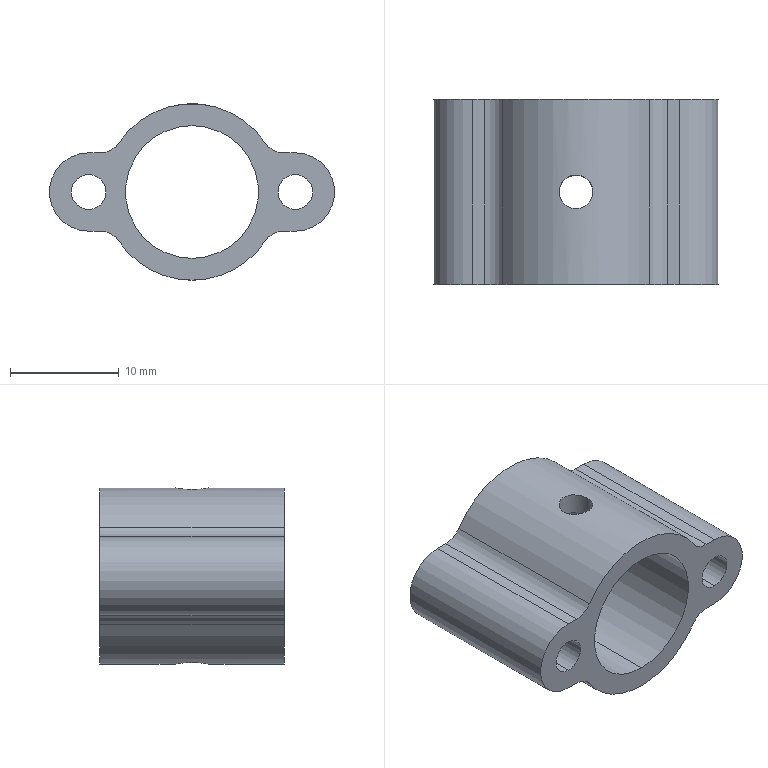Part | SolidWorks | features Extrusion 1, Fillet 1, ICE 1 | 1 solid | 25 faces | box 26.2 x 17 x 16.2 mm | volume 2329 mm3 | cylinder 19 | plane 6 | commonest cylinder face diameters 3.1 x4 3.2 x4 4 x4 16.2 x3 7.2 x2 12.2 x2
STEP:
#1=CARTESIAN_POINT('',(-1.55,8.5,-7.95));
#2=VERTEX_POINT('',#1);
#3=CARTESIAN_POINT('',(0.,6.95,-8.1));
#4=VERTEX_POINT('',#3);
#5=CARTESIAN_POINT('',(-1.55,8.5,-7.95));
#6=CARTESIAN_POINT('',(-1.55,8.398,-7.95));
#7=CARTESIAN_POINT('',(-1.54,8.297,-7.952));
#8=CARTESIAN_POINT('',(-1.5,8.098,-7.96));
#9=CARTESIAN_POINT('',(-1.471,8.,-7.965));
#10=CARTESIAN_POINT('',(-1.393,7.812,-7.979));
#11=CARTESIAN_POINT('',(-1.345,7.724,-7.988));
#12=CARTESIAN_POINT('',(-1.233,7.555,-8.006));
#13=CARTESIAN_POINT('',(-1.168,7.476,-8.016));
#14=CARTESIAN_POINT('',(-0.9541,7.262,-8.045));
#15=CARTESIAN_POINT('',(-0.7816,7.146,-8.064));
#16=CARTESIAN_POINT('',(-0.409,6.991,-8.092));
#17=CARTESIAN_POINT('',(-0.2052,6.95,-8.1));
#18=CARTESIAN_POINT('',(0.,6.95,-8.1));
#19=B_SPLINE_CURVE_WITH_KNOTS('',3,(#5,#6,#7,#8,#9,#10,#11,#12,#13,#14,#15,#16,#17,#18),.UNSPECIFIED.,.F.,.F.,(4,2,2,2,2,2,4),(0.007286,0.007589,0.007893,0.008196,0.0085,0.009106,0.009713),.UNSPECIFIED.);
#20=EDGE_CURVE('',#2,#4,#19,.T.);
#21=ORIENTED_EDGE('',*,*,#20,.F.);
#22=CARTESIAN_POINT('',(-1.55,8.5,-5.9));
#23=VERTEX_POINT('',#22);
#24=CARTESIAN_POINT('',(-1.55,8.5,-8.1));
#25=DIRECTION('',(0.,0.,1.));
#26=VECTOR('',#25,1000.);
#27=LINE('',#24,#26);
#28=EDGE_CURVE('',#2,#23,#27,.T.);
#29=ORIENTED_EDGE('',*,*,#28,.T.);
#30=CARTESIAN_POINT('',(0.,6.95,-6.1));
#31=VERTEX_POINT('',#30);
#32=CARTESIAN_POINT('',(-1.55,8.5,-5.9));
#33=CARTESIAN_POINT('',(-1.55,8.398,-5.9));
#34=CARTESIAN_POINT('',(-1.54,8.295,-5.903));
#35=CARTESIAN_POINT('',(-1.5,8.096,-5.913));
#36=CARTESIAN_POINT('',(-1.47,7.999,-5.92));
#37=CARTESIAN_POINT('',(-1.353,7.717,-5.949));
#38=CARTESIAN_POINT('',(-1.239,7.547,-5.975));
#39=CARTESIAN_POINT('',(-1.024,7.332,-6.014));
#40=CARTESIAN_POINT('',(-0.9459,7.268,-6.027));
#41=CARTESIAN_POINT('',(-0.7784,7.156,-6.051));
#42=CARTESIAN_POINT('',(-0.6876,7.107,-6.062));
#43=CARTESIAN_POINT('',(-0.5005,7.03,-6.08));
#44=CARTESIAN_POINT('',(-0.4039,7.,-6.087));
#45=CARTESIAN_POINT('',(-0.2043,6.96,-6.097));
#46=CARTESIAN_POINT('',(-0.1014,6.95,-6.1));
#47=CARTESIAN_POINT('',(0.,6.95,-6.1));
#48=B_SPLINE_CURVE_WITH_KNOTS('',3,(#32,#33,#34,#35,#36,#37,#38,#39,#40,#41,#42,#43,#44,#45,#46,#47),.UNSPECIFIED.,.F.,.F.,(4,2,2,2,2,2,2,4),(0.002434,0.002738,0.003042,0.00365,0.003954,0.004258,0.004562,0.004866),.UNSPECIFIED.);
#49=EDGE_CURVE('',#23,#31,#48,.T.);
#50=ORIENTED_EDGE('',*,*,#49,.T.);
#51=CARTESIAN_POINT('',(1.55,8.5,-5.9));
#52=VERTEX_POINT('',#51);
#53=CARTESIAN_POINT('',(0.,6.95,-6.1));
#54=CARTESIAN_POINT('',(0.2028,6.95,-6.1));
#55=CARTESIAN_POINT('',(0.4076,6.991,-6.089));
#56=CARTESIAN_POINT('',(0.6877,7.107,-6.062));
#57=CARTESIAN_POINT('',(0.7783,7.156,-6.051));
#58=CARTESIAN_POINT('',(0.9465,7.268,-6.027));
#59=CARTESIAN_POINT('',(1.024,7.332,-6.014));
#60=CARTESIAN_POINT('',(1.167,7.475,-5.988));
#61=CARTESIAN_POINT('',(1.232,7.554,-5.975));
#62=CARTESIAN_POINT('',(1.344,7.722,-5.95));
#63=CARTESIAN_POINT('',(1.392,7.811,-5.939));
#64=CARTESIAN_POINT('',(1.51,8.094,-5.911));
#65=CARTESIAN_POINT('',(1.55,8.296,-5.9));
#66=CARTESIAN_POINT('',(1.55,8.5,-5.9));
#67=B_SPLINE_CURVE_WITH_KNOTS('',3,(#53,#54,#55,#56,#57,#58,#59,#60,#61,#62,#63,#64,#65,#66),.UNSPECIFIED.,.F.,.F.,(4,2,2,2,2,2,4),(0.004866,0.005474,0.005778,0.006082,0.006387,0.006691,0.007299),.UNSPECIFIED.);
#68=EDGE_CURVE('',#31,#52,#67,.T.);
#69=ORIENTED_EDGE('',*,*,#68,.T.);
#70=CARTESIAN_POINT('',(1.55,8.5,-7.95));
#71=VERTEX_POINT('',#70);
#72=CARTESIAN_POINT('',(1.55,8.5,-8.1));
#73=DIRECTION('',(0.,0.,1.));
#74=VECTOR('',#73,1000.);
#75=LINE('',#72,#74);
#76=EDGE_CURVE('',#71,#52,#75,.T.);
#77=ORIENTED_EDGE('',*,*,#76,.F.);
#78=CARTESIAN_POINT('',(0.,6.95,-8.1));
#79=CARTESIAN_POINT('',(0.1027,6.95,-8.1));
#80=CARTESIAN_POINT('',(0.2036,6.96,-8.098));
#81=CARTESIAN_POINT('',(0.4021,7.,-8.091));
#82=CARTESIAN_POINT('',(0.5007,7.03,-8.085));
#83=CARTESIAN_POINT('',(0.6884,7.108,-8.071));
#84=CARTESIAN_POINT('',(0.7773,7.155,-8.063));
#85=CARTESIAN_POINT('',(0.9457,7.268,-8.045));
#86=CARTESIAN_POINT('',(1.025,7.333,-8.035));
#87=CARTESIAN_POINT('',(1.239,7.547,-8.006));
#88=CARTESIAN_POINT('',(1.354,7.72,-7.986));
#89=CARTESIAN_POINT('',(1.509,8.093,-7.959));
#90=CARTESIAN_POINT('',(1.55,8.297,-7.95));
#91=CARTESIAN_POINT('',(1.55,8.5,-7.95));
#92=B_SPLINE_CURVE_WITH_KNOTS('',3,(#78,#79,#80,#81,#82,#83,#84,#85,#86,#87,#88,#89,#90,#91),.UNSPECIFIED.,.F.,.F.,(4,2,2,2,2,2,4),(0.,0.0003037,0.0006073,0.000911,0.001215,0.001822,0.002429),.UNSPECIFIED.);
#93=EDGE_CURVE('',#4,#71,#92,.T.);
#94=ORIENTED_EDGE('',*,*,#93,.F.);
#95=EDGE_LOOP('',(#21,#29,#50,#69,#77,#94));
#96=FACE_OUTER_BOUND('',#95,.T.);
#97=CARTESIAN_POINT('',(0.,8.5,-8.1));
#98=DIRECTION('',(0.,0.,1.));
#99=DIRECTION('',(1.,0.,0.));
#100=AXIS2_PLACEMENT_3D('',#97,#98,#99);
#101=CYLINDRICAL_SURFACE('',#100,1.55);
#102=ADVANCED_FACE('',(#96),#101,.F.);
#103=CARTESIAN_POINT('',(0.,6.95,6.1));
#104=VERTEX_POINT('',#103);
#105=CARTESIAN_POINT('',(-1.55,8.5,5.9));
#106=VERTEX_POINT('',#105);
#107=CARTESIAN_POINT('',(0.,6.95,6.1));
#108=CARTESIAN_POINT('',(-0.1016,6.95,6.1));
#109=CARTESIAN_POINT('',(-0.2047,6.96,6.097));
#110=CARTESIAN_POINT('',(-0.4038,7.,6.087));
#111=CARTESIAN_POINT('',(-0.5006,7.03,6.08));
#112=CARTESIAN_POINT('',(-0.7828,7.147,6.053));
#113=CARTESIAN_POINT('',(-0.9531,7.261,6.027));
#114=CARTESIAN_POINT('',(-1.168,7.476,5.988));
#115=CARTESIAN_POINT('',(-1.232,7.554,5.975));
#116=CARTESIAN_POINT('',(-1.344,7.722,5.95));
#117=CARTESIAN_POINT('',(-1.393,7.812,5.939));
#118=CARTESIAN_POINT('',(-1.47,7.999,5.92));
#119=CARTESIAN_POINT('',(-1.5,8.096,5.913));
#120=CARTESIAN_POINT('',(-1.54,8.296,5.902));
#121=CARTESIAN_POINT('',(-1.55,8.399,5.9));
#122=CARTESIAN_POINT('',(-1.55,8.5,5.9));
#123=B_SPLINE_CURVE_WITH_KNOTS('',3,(#107,#108,#109,#110,#111,#112,#113,#114,#115,#116,#117,#118,#119,#120,#121,#122),.UNSPECIFIED.,.F.,.F.,(4,2,2,2,2,2,2,4),(0.002434,0.002738,0.003042,0.00365,0.003954,0.004258,0.004562,0.004866),.UNSPECIFIED.);
#124=EDGE_CURVE('',#104,#106,#123,.T.);
#125=ORIENTED_EDGE('',*,*,#124,.T.);
#126=CARTESIAN_POINT('',(-1.55,8.5,7.95));
#127=VERTEX_POINT('',#126);
#128=CARTESIAN_POINT('',(-1.55,8.5,-8.1));
#129=DIRECTION('',(0.,0.,1.));
#130=VECTOR('',#129,1000.);
#131=LINE('',#128,#130);
#132=EDGE_CURVE('',#106,#127,#131,.T.);
#133=ORIENTED_EDGE('',*,*,#132,.T.);
#134=CARTESIAN_POINT('',(1.55,8.5,7.95));
#135=VERTEX_POINT('',#134);
#136=CARTESIAN_POINT('',(1.55,8.5,7.95));
#137=CARTESIAN_POINT('',(1.55,8.397,7.95));
#138=CARTESIAN_POINT('',(1.54,8.296,7.952));
#139=CARTESIAN_POINT('',(1.5,8.098,7.96));
#140=CARTESIAN_POINT('',(1.47,7.999,7.966));
#141=CARTESIAN_POINT('',(1.393,7.812,7.979));
#142=CARTESIAN_POINT('',(1.345,7.723,7.988));
#143=CARTESIAN_POINT('',(1.232,7.555,8.006));
#144=CARTESIAN_POINT('',(1.167,7.475,8.016));
#145=CARTESIAN_POINT('',(0.9531,7.261,8.045));
#146=CARTESIAN_POINT('',(0.7805,7.146,8.064));
#147=CARTESIAN_POINT('',(0.4076,6.991,8.092));
#148=CARTESIAN_POINT('',(0.2033,6.95,8.1));
#149=CARTESIAN_POINT('',(-0.1008,6.95,8.1));
#150=CARTESIAN_POINT('',(-0.2037,6.96,8.098));
#151=CARTESIAN_POINT('',(-0.4027,7.,8.091));
#152=CARTESIAN_POINT('',(-0.4995,7.029,8.085));
#153=CARTESIAN_POINT('',(-0.7814,7.146,8.064));
#154=CARTESIAN_POINT('',(-0.952,7.26,8.045));
#155=CARTESIAN_POINT('',(-1.168,7.476,8.016));
#156=CARTESIAN_POINT('',(-1.232,7.554,8.006));
#157=CARTESIAN_POINT('',(-1.344,7.722,7.988));
#158=CARTESIAN_POINT('',(-1.393,7.813,7.979));
#159=CARTESIAN_POINT('',(-1.471,8.,7.965));
#160=CARTESIAN_POINT('',(-1.5,8.097,7.96));
#161=CARTESIAN_POINT('',(-1.54,8.296,7.952));
#162=CARTESIAN_POINT('',(-1.55,8.399,7.95));
#163=CARTESIAN_POINT('',(-1.55,8.5,7.95));
#164=B_SPLINE_CURVE_WITH_KNOTS('',3,(#136,#137,#138,#139,#140,#141,#142,#143,#144,#145,#146,#147,#148,#149,#150,#151,#152,#153,#154,#155,#156,#157,#158,#159,#160,#161,#162,#163),.UNSPECIFIED.,.F.,.F.,(4,2,2,2,2,2,2,2,2,2,2,2,2,4),(0.,0.0003036,0.0006072,0.0009107,0.001214,0.001821,0.002429,0.002732,0.003036,0.003643,0.003946,0.00425,0.004554,0.004857),.UNSPECIFIED.);
#165=EDGE_CURVE('',#135,#127,#164,.T.);
#166=ORIENTED_EDGE('',*,*,#165,.F.);
#167=CARTESIAN_POINT('',(1.55,8.5,5.9));
#168=VERTEX_POINT('',#167);
#169=CARTESIAN_POINT('',(1.55,8.5,-8.1));
#170=DIRECTION('',(0.,0.,1.));
#171=VECTOR('',#170,1000.);
#172=LINE('',#169,#171);
#173=EDGE_CURVE('',#168,#135,#172,.T.);
#174=ORIENTED_EDGE('',*,*,#173,.F.);
#175=CARTESIAN_POINT('',(1.55,8.5,5.9));
#176=CARTESIAN_POINT('',(1.55,8.397,5.9));
#177=CARTESIAN_POINT('',(1.54,8.296,5.902));
#178=CARTESIAN_POINT('',(1.5,8.097,5.913));
#179=CARTESIAN_POINT('',(1.47,7.999,5.92));
#180=CARTESIAN_POINT('',(1.392,7.811,5.939));
#181=CARTESIAN_POINT('',(1.345,7.722,5.95));
#182=CARTESIAN_POINT('',(1.232,7.554,5.975));
#183=CARTESIAN_POINT('',(1.167,7.475,5.988));
#184=CARTESIAN_POINT('',(0.9531,7.261,6.027));
#185=CARTESIAN_POINT('',(0.7807,7.146,6.053));
#186=CARTESIAN_POINT('',(0.4078,6.991,6.089));
#187=CARTESIAN_POINT('',(0.2032,6.95,6.1));
#188=CARTESIAN_POINT('',(0.,6.95,6.1));
#189=B_SPLINE_CURVE_WITH_KNOTS('',3,(#175,#176,#177,#178,#179,#180,#181,#182,#183,#184,#185,#186,#187,#188),.UNSPECIFIED.,.F.,.F.,(4,2,2,2,2,2,4),(0.,0.0003042,0.0006084,0.0009126,0.001217,0.001825,0.002434),.UNSPECIFIED.);
#190=EDGE_CURVE('',#168,#104,#189,.T.);
#191=ORIENTED_EDGE('',*,*,#190,.T.);
#192=EDGE_LOOP('',(#125,#133,#166,#174,#191));
#193=FACE_OUTER_BOUND('',#192,.T.);
#194=CARTESIAN_POINT('',(0.,8.5,-8.1));
#195=DIRECTION('',(0.,0.,1.));
#196=DIRECTION('',(1.,0.,0.));
#197=AXIS2_PLACEMENT_3D('',#194,#195,#196);
#198=CYLINDRICAL_SURFACE('',#197,1.55);
#199=ADVANCED_FACE('',(#193),#198,.F.);
#200=CARTESIAN_POINT('',(-9.5,17.,-1.6));
#201=VERTEX_POINT('',#200);
#202=CARTESIAN_POINT('',(-9.5,17.,1.6));
#203=VERTEX_POINT('',#202);
#204=CARTESIAN_POINT('',(-9.5,17.,0.));
#205=DIRECTION('',(0.,1.,0.));
#206=DIRECTION('',(0.,0.,-1.));
#207=AXIS2_PLACEMENT_3D('',#204,#205,#206);
#208=CIRCLE('',#207,1.6);
#209=EDGE_CURVE('',#201,#203,#208,.T.);
#210=ORIENTED_EDGE('',*,*,#209,.T.);
#211=CARTESIAN_POINT('',(-9.5,0.,1.6));
#212=VERTEX_POINT('',#211);
#213=CARTESIAN_POINT('',(-9.5,17.,1.6));
#214=DIRECTION('',(0.,-1.,0.));
#215=VECTOR('',#214,1000.);
#216=LINE('',#213,#215);
#217=EDGE_CURVE('',#203,#212,#216,.T.);
#218=ORIENTED_EDGE('',*,*,#217,.T.);
#219=CARTESIAN_POINT('',(-9.5,0.,-1.6));
#220=VERTEX_POINT('',#219);
#221=CARTESIAN_POINT('',(-9.5,0.,0.));
#222=DIRECTION('',(0.,1.,0.));
#223=DIRECTION('',(0.,0.,-1.));
#224=AXIS2_PLACEMENT_3D('',#221,#222,#223);
#225=CIRCLE('',#224,1.6);
#226=EDGE_CURVE('',#220,#212,#225,.T.);
#227=ORIENTED_EDGE('',*,*,#226,.F.);
#228=CARTESIAN_POINT('',(-9.5,17.,-1.6));
#229=DIRECTION('',(0.,-1.,0.));
#230=VECTOR('',#229,1000.);
#231=LINE('',#228,#230);
#232=EDGE_CURVE('',#201,#220,#231,.T.);
#233=ORIENTED_EDGE('',*,*,#232,.F.);
#234=EDGE_LOOP('',(#210,#218,#227,#233));
#235=FACE_OUTER_BOUND('',#234,.T.);
#236=CARTESIAN_POINT('',(-9.5,17.,0.));
#237=DIRECTION('',(0.,-1.,0.));
#238=DIRECTION('',(0.,0.,-1.));
#239=AXIS2_PLACEMENT_3D('',#236,#237,#238);
#240=CYLINDRICAL_SURFACE('',#239,1.6);
#241=ADVANCED_FACE('',(#235),#240,.F.);
#242=CARTESIAN_POINT('',(9.5,17.,-1.6));
#243=VERTEX_POINT('',#242);
#244=CARTESIAN_POINT('',(9.5,17.,1.6));
#245=VERTEX_POINT('',#244);
#246=CARTESIAN_POINT('',(9.5,17.,0.));
#247=DIRECTION('',(0.,1.,0.));
#248=DIRECTION('',(0.,0.,1.));
#249=AXIS2_PLACEMENT_3D('',#246,#247,#248);
#250=CIRCLE('',#249,1.6);
#251=EDGE_CURVE('',#243,#245,#250,.T.);
#252=ORIENTED_EDGE('',*,*,#251,.T.);
#253=CARTESIAN_POINT('',(9.5,0.,1.6));
#254=VERTEX_POINT('',#253);
#255=CARTESIAN_POINT('',(9.5,17.,1.6));
#256=DIRECTION('',(0.,-1.,0.));
#257=VECTOR('',#256,1000.);
#258=LINE('',#255,#257);
#259=EDGE_CURVE('',#245,#254,#258,.T.);
#260=ORIENTED_EDGE('',*,*,#259,.T.);
#261=CARTESIAN_POINT('',(9.5,0.,-1.6));
#262=VERTEX_POINT('',#261);
#263=CARTESIAN_POINT('',(9.5,0.,0.));
#264=DIRECTION('',(0.,1.,0.));
#265=DIRECTION('',(0.,0.,1.));
#266=AXIS2_PLACEMENT_3D('',#263,#264,#265);
#267=CIRCLE('',#266,1.6);
#268=EDGE_CURVE('',#262,#254,#267,.T.);
#269=ORIENTED_EDGE('',*,*,#268,.F.);
#270=CARTESIAN_POINT('',(9.5,17.,-1.6));
#271=DIRECTION('',(0.,-1.,0.));
#272=VECTOR('',#271,1000.);
#273=LINE('',#270,#272);
#274=EDGE_CURVE('',#243,#262,#273,.T.);
#275=ORIENTED_EDGE('',*,*,#274,.F.);
#276=EDGE_LOOP('',(#252,#260,#269,#275));
#277=FACE_OUTER_BOUND('',#276,.T.);
#278=CARTESIAN_POINT('',(9.5,17.,0.));
#279=DIRECTION('',(0.,-1.,0.));
#280=DIRECTION('',(0.,0.,-1.));
#281=AXIS2_PLACEMENT_3D('',#278,#279,#280);
#282=CYLINDRICAL_SURFACE('',#281,1.6);
#283=ADVANCED_FACE('',(#277),#282,.F.);
#284=CARTESIAN_POINT('',(0.,17.,-6.1));
#285=VERTEX_POINT('',#284);
#286=CARTESIAN_POINT('',(0.,17.,6.1));
#287=VERTEX_POINT('',#286);
#288=CARTESIAN_POINT('',(0.,17.,0.));
#289=DIRECTION('',(0.,1.,0.));
#290=DIRECTION('',(0.,0.,1.));
#291=AXIS2_PLACEMENT_3D('',#288,#289,#290);
#292=CIRCLE('',#291,6.1);
#293=EDGE_CURVE('',#285,#287,#292,.T.);
#294=ORIENTED_EDGE('',*,*,#293,.T.);
#295=CARTESIAN_POINT('',(0.,10.05,6.1));
#296=VERTEX_POINT('',#295);
#297=CARTESIAN_POINT('',(0.,17.,6.1));
#298=DIRECTION('',(0.,-1.,0.));
#299=VECTOR('',#298,1000.);
#300=LINE('',#297,#299);
#301=EDGE_CURVE('',#287,#296,#300,.T.);
#302=ORIENTED_EDGE('',*,*,#301,.T.);
#303=CARTESIAN_POINT('',(-1.55,8.5,5.9));
#304=CARTESIAN_POINT('',(-1.55,8.703,5.9));
#305=CARTESIAN_POINT('',(-1.509,8.908,5.911));
#306=CARTESIAN_POINT('',(-1.393,9.188,5.939));
#307=CARTESIAN_POINT('',(-1.344,9.278,5.95));
#308=CARTESIAN_POINT('',(-1.232,9.446,5.975));
#309=CARTESIAN_POINT('',(-1.168,9.524,5.988));
#310=CARTESIAN_POINT('',(-1.025,9.667,6.014));
#311=CARTESIAN_POINT('',(-0.9456,9.732,6.027));
#312=CARTESIAN_POINT('',(-0.7782,9.844,6.051));
#313=CARTESIAN_POINT('',(-0.6893,9.892,6.062));
#314=CARTESIAN_POINT('',(-0.4063,10.01,6.089));
#315=CARTESIAN_POINT('',(-0.2045,10.05,6.1));
#316=CARTESIAN_POINT('',(0.,10.05,6.1));
#317=B_SPLINE_CURVE_WITH_KNOTS('',3,(#303,#304,#305,#306,#307,#308,#309,#310,#311,#312,#313,#314,#315,#316),.UNSPECIFIED.,.F.,.F.,(4,2,2,2,2,2,4),(0.004866,0.005474,0.005778,0.006082,0.006386,0.006691,0.007299),.UNSPECIFIED.);
#318=EDGE_CURVE('',#106,#296,#317,.T.);
#319=ORIENTED_EDGE('',*,*,#318,.F.);
#320=ORIENTED_EDGE('',*,*,#124,.F.);
#321=CARTESIAN_POINT('',(0.,0.,6.1));
#322=VERTEX_POINT('',#321);
#323=CARTESIAN_POINT('',(0.,17.,6.1));
#324=DIRECTION('',(0.,-1.,0.));
#325=VECTOR('',#324,1000.);
#326=LINE('',#323,#325);
#327=EDGE_CURVE('',#104,#322,#326,.T.);
#328=ORIENTED_EDGE('',*,*,#327,.T.);
#329=CARTESIAN_POINT('',(0.,0.,-6.1));
#330=VERTEX_POINT('',#329);
#331=CARTESIAN_POINT('',(0.,0.,0.));
#332=DIRECTION('',(0.,1.,0.));
#333=DIRECTION('',(0.,0.,1.));
#334=AXIS2_PLACEMENT_3D('',#331,#332,#333);
#335=CIRCLE('',#334,6.1);
#336=EDGE_CURVE('',#330,#322,#335,.T.);
#337=ORIENTED_EDGE('',*,*,#336,.F.);
#338=CARTESIAN_POINT('',(0.,17.,-6.1));
#339=DIRECTION('',(0.,-1.,0.));
#340=VECTOR('',#339,1000.);
#341=LINE('',#338,#340);
#342=EDGE_CURVE('',#31,#330,#341,.T.);
#343=ORIENTED_EDGE('',*,*,#342,.F.);
#344=ORIENTED_EDGE('',*,*,#49,.F.);
#345=CARTESIAN_POINT('',(0.,10.05,-6.1));
#346=VERTEX_POINT('',#345);
#347=CARTESIAN_POINT('',(0.,10.05,-6.1));
#348=CARTESIAN_POINT('',(-0.1029,10.05,-6.1));
#349=CARTESIAN_POINT('',(-0.204,10.04,-6.097));
#350=CARTESIAN_POINT('',(-0.4027,10.,-6.088));
#351=CARTESIAN_POINT('',(-0.5015,9.97,-6.08));
#352=CARTESIAN_POINT('',(-0.689,9.892,-6.062));
#353=CARTESIAN_POINT('',(-0.7779,9.844,-6.051));
#354=CARTESIAN_POINT('',(-0.9461,9.732,-6.027));
#355=CARTESIAN_POINT('',(-1.025,9.667,-6.014));
#356=CARTESIAN_POINT('',(-1.239,9.453,-5.975));
#357=CARTESIAN_POINT('',(-1.354,9.281,-5.948));
#358=CARTESIAN_POINT('',(-1.509,8.908,-5.911));
#359=CARTESIAN_POINT('',(-1.55,8.703,-5.9));
#360=CARTESIAN_POINT('',(-1.55,8.5,-5.9));
#361=B_SPLINE_CURVE_WITH_KNOTS('',3,(#347,#348,#349,#350,#351,#352,#353,#354,#355,#356,#357,#358,#359,#360),.UNSPECIFIED.,.F.,.F.,(4,2,2,2,2,2,4),(0.,0.0003042,0.0006084,0.0009126,0.001217,0.001825,0.002434),.UNSPECIFIED.);
#362=EDGE_CURVE('',#346,#23,#361,.T.);
#363=ORIENTED_EDGE('',*,*,#362,.F.);
#364=CARTESIAN_POINT('',(0.,17.,-6.1));
#365=DIRECTION('',(0.,-1.,0.));
#366=VECTOR('',#365,1000.);
#367=LINE('',#364,#366);
#368=EDGE_CURVE('',#285,#346,#367,.T.);
#369=ORIENTED_EDGE('',*,*,#368,.F.);
#370=EDGE_LOOP('',(#294,#302,#319,#320,#328,#337,#343,#344,#363,#369));
#371=FACE_OUTER_BOUND('',#370,.T.);
#372=CARTESIAN_POINT('',(0.,17.,0.));
#373=DIRECTION('',(0.,-1.,0.));
#374=DIRECTION('',(0.,0.,-1.));
#375=AXIS2_PLACEMENT_3D('',#372,#373,#374);
#376=CYLINDRICAL_SURFACE('',#375,6.1);
#377=ADVANCED_FACE('',(#371),#376,.F.);
#378=CARTESIAN_POINT('',(0.,17.,-8.1));
#379=VERTEX_POINT('',#378);
#380=CARTESIAN_POINT('',(-6.741,17.,-4.491));
#381=VERTEX_POINT('',#380);
#382=CARTESIAN_POINT('',(0.,17.,0.));
#383=DIRECTION('',(0.,1.,0.));
#384=DIRECTION('',(0.,0.,1.));
#385=AXIS2_PLACEMENT_3D('',#382,#383,#384);
#386=CIRCLE('',#385,8.1);
#387=EDGE_CURVE('',#379,#381,#386,.T.);
#388=ORIENTED_EDGE('',*,*,#387,.F.);
#389=CARTESIAN_POINT('',(0.,10.05,-8.1));
#390=VERTEX_POINT('',#389);
#391=CARTESIAN_POINT('',(0.,17.,-8.1));
#392=DIRECTION('',(0.,-1.,0.));
#393=VECTOR('',#392,1000.);
#394=LINE('',#391,#393);
#395=EDGE_CURVE('',#379,#390,#394,.T.);
#396=ORIENTED_EDGE('',*,*,#395,.T.);
#397=CARTESIAN_POINT('',(0.,10.05,-8.1));
#398=CARTESIAN_POINT('',(-0.2026,10.05,-8.1));
#399=CARTESIAN_POINT('',(-0.407,10.009,-8.092));
#400=CARTESIAN_POINT('',(-0.7803,9.854,-8.064));
#401=CARTESIAN_POINT('',(-0.9527,9.739,-8.045));
#402=CARTESIAN_POINT('',(-1.167,9.525,-8.016));
#403=CARTESIAN_POINT('',(-1.232,9.445,-8.006));
#404=CARTESIAN_POINT('',(-1.345,9.277,-7.988));
#405=CARTESIAN_POINT('',(-1.392,9.188,-7.98));
#406=CARTESIAN_POINT('',(-1.51,8.906,-7.958));
#407=CARTESIAN_POINT('',(-1.55,8.705,-7.95));
#408=CARTESIAN_POINT('',(-1.55,8.5,-7.95));
#409=B_SPLINE_CURVE_WITH_KNOTS('',3,(#397,#398,#399,#400,#401,#402,#403,#404,#405,#406,#407,#408),.UNSPECIFIED.,.F.,.F.,(4,2,2,2,2,4),(0.004857,0.005464,0.006072,0.006375,0.006679,0.007286),.UNSPECIFIED.);
#410=EDGE_CURVE('',#390,#2,#409,.T.);
#411=ORIENTED_EDGE('',*,*,#410,.T.);
#412=ORIENTED_EDGE('',*,*,#20,.T.);
#413=CARTESIAN_POINT('',(0.,0.,-8.1));
#414=VERTEX_POINT('',#413);
#415=CARTESIAN_POINT('',(0.,17.,-8.1));
#416=DIRECTION('',(0.,-1.,0.));
#417=VECTOR('',#416,1000.);
#418=LINE('',#415,#417);
#419=EDGE_CURVE('',#4,#414,#418,.T.);
#420=ORIENTED_EDGE('',*,*,#419,.T.);
#421=CARTESIAN_POINT('',(-6.741,0.,-4.491));
#422=VERTEX_POINT('',#421);
#423=CARTESIAN_POINT('',(0.,0.,0.));
#424=DIRECTION('',(0.,1.,0.));
#425=DIRECTION('',(0.,0.,1.));
#426=AXIS2_PLACEMENT_3D('',#423,#424,#425);
#427=CIRCLE('',#426,8.1);
#428=EDGE_CURVE('',#414,#422,#427,.T.);
#429=ORIENTED_EDGE('',*,*,#428,.T.);
#430=CARTESIAN_POINT('',(-6.741,17.,-4.491));
#431=DIRECTION('',(0.,1.,0.));
#432=VECTOR('',#431,1000.);
#433=LINE('',#430,#432);
#434=EDGE_CURVE('',#422,#381,#433,.T.);
#435=ORIENTED_EDGE('',*,*,#434,.T.);
#436=EDGE_LOOP('',(#388,#396,#411,#412,#420,#429,#435));
#437=FACE_OUTER_BOUND('',#436,.T.);
#438=CARTESIAN_POINT('',(0.,17.,0.));
#439=DIRECTION('',(0.,-1.,0.));
#440=DIRECTION('',(0.,0.,-1.));
#441=AXIS2_PLACEMENT_3D('',#438,#439,#440);
#442=CYLINDRICAL_SURFACE('',#441,8.1);
#443=ADVANCED_FACE('',(#437),#442,.T.);
#444=CARTESIAN_POINT('',(-9.5,17.,-3.6));
#445=VERTEX_POINT('',#444);
#446=CARTESIAN_POINT('',(-9.5,17.,3.6));
#447=VERTEX_POINT('',#446);
#448=CARTESIAN_POINT('',(-9.5,17.,0.));
#449=DIRECTION('',(0.,1.,0.));
#450=DIRECTION('',(0.,0.,-1.));
#451=AXIS2_PLACEMENT_3D('',#448,#449,#450);
#452=CIRCLE('',#451,3.6);
#453=EDGE_CURVE('',#445,#447,#452,.T.);
#454=ORIENTED_EDGE('',*,*,#453,.T.);
#455=CARTESIAN_POINT('',(-8.405,17.,3.6));
#456=VERTEX_POINT('',#455);
#457=CARTESIAN_POINT('',(-9.5,17.,3.6));
#458=DIRECTION('',(1.,0.,0.));
#459=VECTOR('',#458,1000.);
#460=LINE('',#457,#459);
#461=EDGE_CURVE('',#447,#456,#460,.T.);
#462=ORIENTED_EDGE('',*,*,#461,.T.);
#463=CARTESIAN_POINT('',(-6.741,17.,4.491));
#464=VERTEX_POINT('',#463);
#465=CARTESIAN_POINT('',(-8.405,17.,5.6));
#466=DIRECTION('',(0.,-1.,0.));
#467=DIRECTION('',(0.,0.,-1.));
#468=AXIS2_PLACEMENT_3D('',#465,#466,#467);
#469=CIRCLE('',#468,2.);
#470=EDGE_CURVE('',#456,#464,#469,.T.);
#471=ORIENTED_EDGE('',*,*,#470,.T.);
#472=CARTESIAN_POINT('',(6.741,17.,4.491));
#473=VERTEX_POINT('',#472);
#474=CARTESIAN_POINT('',(0.,17.,0.));
#475=DIRECTION('',(0.,1.,0.));
#476=DIRECTION('',(0.,0.,1.));
#477=AXIS2_PLACEMENT_3D('',#474,#475,#476);
#478=CIRCLE('',#477,8.1);
#479=EDGE_CURVE('',#464,#473,#478,.T.);
#480=ORIENTED_EDGE('',*,*,#479,.T.);
#481=CARTESIAN_POINT('',(8.405,17.,3.6));
#482=VERTEX_POINT('',#481);
#483=CARTESIAN_POINT('',(8.405,17.,5.6));
#484=DIRECTION('',(0.,-1.,0.));
#485=DIRECTION('',(0.,0.,-1.));
#486=AXIS2_PLACEMENT_3D('',#483,#484,#485);
#487=CIRCLE('',#486,2.);
#488=EDGE_CURVE('',#473,#482,#487,.T.);
#489=ORIENTED_EDGE('',*,*,#488,.T.);
#490=CARTESIAN_POINT('',(9.5,17.,3.6));
#491=VERTEX_POINT('',#490);
#492=CARTESIAN_POINT('',(9.5,17.,3.6));
#493=DIRECTION('',(1.,0.,0.));
#494=VECTOR('',#493,1000.);
#495=LINE('',#492,#494);
#496=EDGE_CURVE('',#482,#491,#495,.T.);
#497=ORIENTED_EDGE('',*,*,#496,.T.);
#498=CARTESIAN_POINT('',(9.5,17.,-3.6));
#499=VERTEX_POINT('',#498);
#500=CARTESIAN_POINT('',(9.5,17.,0.));
#501=DIRECTION('',(0.,1.,0.));
#502=DIRECTION('',(0.,0.,1.));
#503=AXIS2_PLACEMENT_3D('',#500,#501,#502);
#504=CIRCLE('',#503,3.6);
#505=EDGE_CURVE('',#491,#499,#504,.T.);
#506=ORIENTED_EDGE('',*,*,#505,.T.);
#507=CARTESIAN_POINT('',(8.405,17.,-3.6));
#508=VERTEX_POINT('',#507);
#509=CARTESIAN_POINT('',(9.5,17.,-3.6));
#510=DIRECTION('',(-1.,0.,0.));
#511=VECTOR('',#510,1000.);
#512=LINE('',#509,#511);
#513=EDGE_CURVE('',#499,#508,#512,.T.);
#514=ORIENTED_EDGE('',*,*,#513,.T.);
#515=CARTESIAN_POINT('',(6.741,17.,-4.491));
#516=VERTEX_POINT('',#515);
#517=CARTESIAN_POINT('',(8.405,17.,-5.6));
#518=DIRECTION('',(0.,-1.,0.));
#519=DIRECTION('',(0.,0.,-1.));
#520=AXIS2_PLACEMENT_3D('',#517,#518,#519);
#521=CIRCLE('',#520,2.);
#522=EDGE_CURVE('',#508,#516,#521,.T.);
#523=ORIENTED_EDGE('',*,*,#522,.T.);
#524=CARTESIAN_POINT('',(0.,17.,0.));
#525=DIRECTION('',(0.,1.,0.));
#526=DIRECTION('',(0.,0.,1.));
#527=AXIS2_PLACEMENT_3D('',#524,#525,#526);
#528=CIRCLE('',#527,8.1);
#529=EDGE_CURVE('',#516,#379,#528,.T.);
#530=ORIENTED_EDGE('',*,*,#529,.T.);
#531=ORIENTED_EDGE('',*,*,#387,.T.);
#532=CARTESIAN_POINT('',(-8.405,17.,-3.6));
#533=VERTEX_POINT('',#532);
#534=CARTESIAN_POINT('',(-8.405,17.,-5.6));
#535=DIRECTION('',(0.,-1.,0.));
#536=DIRECTION('',(0.,0.,-1.));
#537=AXIS2_PLACEMENT_3D('',#534,#535,#536);
#538=CIRCLE('',#537,2.);
#539=EDGE_CURVE('',#381,#533,#538,.T.);
#540=ORIENTED_EDGE('',*,*,#539,.T.);
#541=CARTESIAN_POINT('',(-9.5,17.,-3.6));
#542=DIRECTION('',(-1.,0.,0.));
#543=VECTOR('',#542,1000.);
#544=LINE('',#541,#543);
#545=EDGE_CURVE('',#533,#445,#544,.T.);
#546=ORIENTED_EDGE('',*,*,#545,.T.);
#547=EDGE_LOOP('',(#454,#462,#471,#480,#489,#497,#506,#514,#523,#530,#531,#540,#546));
#548=FACE_OUTER_BOUND('',#547,.T.);
#549=ORIENTED_EDGE('',*,*,#293,.F.);
#550=CARTESIAN_POINT('',(0.,17.,0.));
#551=DIRECTION('',(0.,1.,0.));
#552=DIRECTION('',(0.,0.,1.));
#553=AXIS2_PLACEMENT_3D('',#550,#551,#552);
#554=CIRCLE('',#553,6.1);
#555=EDGE_CURVE('',#287,#285,#554,.T.);
#556=ORIENTED_EDGE('',*,*,#555,.F.);
#557=EDGE_LOOP('',(#549,#556));
#558=FACE_BOUND('',#557,.T.);
#559=ORIENTED_EDGE('',*,*,#251,.F.);
#560=CARTESIAN_POINT('',(9.5,17.,0.));
#561=DIRECTION('',(0.,1.,0.));
#562=DIRECTION('',(0.,0.,1.));
#563=AXIS2_PLACEMENT_3D('',#560,#561,#562);
#564=CIRCLE('',#563,1.6);
#565=EDGE_CURVE('',#245,#243,#564,.T.);
#566=ORIENTED_EDGE('',*,*,#565,.F.);
#567=EDGE_LOOP('',(#559,#566));
#568=FACE_BOUND('',#567,.T.);
#569=ORIENTED_EDGE('',*,*,#209,.F.);
#570=CARTESIAN_POINT('',(-9.5,17.,0.));
#571=DIRECTION('',(0.,1.,0.));
#572=DIRECTION('',(0.,0.,-1.));
#573=AXIS2_PLACEMENT_3D('',#570,#571,#572);
#574=CIRCLE('',#573,1.6);
#575=EDGE_CURVE('',#203,#201,#574,.T.);
#576=ORIENTED_EDGE('',*,*,#575,.F.);
#577=EDGE_LOOP('',(#569,#576));
#578=FACE_BOUND('',#577,.T.);
#579=CARTESIAN_POINT('',(-9.5,17.,0.));
#580=DIRECTION('',(0.,-1.,0.));
#581=DIRECTION('',(0.,0.,-1.));
#582=AXIS2_PLACEMENT_3D('',#579,#580,#581);
#583=PLANE('',#582);
#584=ADVANCED_FACE('',(#548,#558,#568,#578),#583,.F.);
#585=ORIENTED_EDGE('',*,*,#268,.T.);
#586=CARTESIAN_POINT('',(9.5,0.,0.));
#587=DIRECTION('',(0.,1.,0.));
#588=DIRECTION('',(0.,0.,1.));
#589=AXIS2_PLACEMENT_3D('',#586,#587,#588);
#590=CIRCLE('',#589,1.6);
#591=EDGE_CURVE('',#254,#262,#590,.T.);
#592=ORIENTED_EDGE('',*,*,#591,.T.);
#593=EDGE_LOOP('',(#585,#592));
#594=FACE_BOUND('',#593,.T.);
#595=CARTESIAN_POINT('',(-9.5,0.,-3.6));
#596=VERTEX_POINT('',#595);
#597=CARTESIAN_POINT('',(-9.5,0.,3.6));
#598=VERTEX_POINT('',#597);
#599=CARTESIAN_POINT('',(-9.5,0.,0.));
#600=DIRECTION('',(0.,1.,0.));
#601=DIRECTION('',(0.,0.,-1.));
#602=AXIS2_PLACEMENT_3D('',#599,#600,#601);
#603=CIRCLE('',#602,3.6);
#604=EDGE_CURVE('',#596,#598,#603,.T.);
#605=ORIENTED_EDGE('',*,*,#604,.F.);
#606=CARTESIAN_POINT('',(-8.405,0.,-3.6));
#607=VERTEX_POINT('',#606);
#608=CARTESIAN_POINT('',(-9.5,0.,-3.6));
#609=DIRECTION('',(-1.,0.,0.));
#610=VECTOR('',#609,1000.);
#611=LINE('',#608,#610);
#612=EDGE_CURVE('',#607,#596,#611,.T.);
#613=ORIENTED_EDGE('',*,*,#612,.F.);
#614=CARTESIAN_POINT('',(-8.405,0.,-5.6));
#615=DIRECTION('',(0.,1.,0.));
#616=DIRECTION('',(0.,0.,-1.));
#617=AXIS2_PLACEMENT_3D('',#614,#615,#616);
#618=CIRCLE('',#617,2.);
#619=EDGE_CURVE('',#607,#422,#618,.T.);
#620=ORIENTED_EDGE('',*,*,#619,.T.);
#621=ORIENTED_EDGE('',*,*,#428,.F.);
#622=CARTESIAN_POINT('',(6.741,0.,-4.491));
#623=VERTEX_POINT('',#622);
#624=CARTESIAN_POINT('',(0.,0.,0.));
#625=DIRECTION('',(0.,1.,0.));
#626=DIRECTION('',(0.,0.,1.));
#627=AXIS2_PLACEMENT_3D('',#624,#625,#626);
#628=CIRCLE('',#627,8.1);
#629=EDGE_CURVE('',#623,#414,#628,.T.);
#630=ORIENTED_EDGE('',*,*,#629,.F.);
#631=CARTESIAN_POINT('',(8.405,0.,-3.6));
#632=VERTEX_POINT('',#631);
#633=CARTESIAN_POINT('',(8.405,0.,-5.6));
#634=DIRECTION('',(0.,1.,0.));
#635=DIRECTION('',(0.,0.,-1.));
#636=AXIS2_PLACEMENT_3D('',#633,#634,#635);
#637=CIRCLE('',#636,2.);
#638=EDGE_CURVE('',#623,#632,#637,.T.);
#639=ORIENTED_EDGE('',*,*,#638,.T.);
#640=CARTESIAN_POINT('',(9.5,0.,-3.6));
#641=VERTEX_POINT('',#640);
#642=CARTESIAN_POINT('',(9.5,0.,-3.6));
#643=DIRECTION('',(-1.,0.,0.));
#644=VECTOR('',#643,1000.);
#645=LINE('',#642,#644);
#646=EDGE_CURVE('',#641,#632,#645,.T.);
#647=ORIENTED_EDGE('',*,*,#646,.F.);
#648=CARTESIAN_POINT('',(9.5,0.,3.6));
#649=VERTEX_POINT('',#648);
#650=CARTESIAN_POINT('',(9.5,0.,0.));
#651=DIRECTION('',(0.,1.,0.));
#652=DIRECTION('',(0.,0.,1.));
#653=AXIS2_PLACEMENT_3D('',#650,#651,#652);
#654=CIRCLE('',#653,3.6);
#655=EDGE_CURVE('',#649,#641,#654,.T.);
#656=ORIENTED_EDGE('',*,*,#655,.F.);
#657=CARTESIAN_POINT('',(8.405,0.,3.6));
#658=VERTEX_POINT('',#657);
#659=CARTESIAN_POINT('',(9.5,0.,3.6));
#660=DIRECTION('',(1.,0.,0.));
#661=VECTOR('',#660,1000.);
#662=LINE('',#659,#661);
#663=EDGE_CURVE('',#658,#649,#662,.T.);
#664=ORIENTED_EDGE('',*,*,#663,.F.);
#665=CARTESIAN_POINT('',(6.741,0.,4.491));
#666=VERTEX_POINT('',#665);
#667=CARTESIAN_POINT('',(8.405,0.,5.6));
#668=DIRECTION('',(0.,1.,0.));
#669=DIRECTION('',(0.,0.,-1.));
#670=AXIS2_PLACEMENT_3D('',#667,#668,#669);
#671=CIRCLE('',#670,2.);
#672=EDGE_CURVE('',#658,#666,#671,.T.);
#673=ORIENTED_EDGE('',*,*,#672,.T.);
#674=CARTESIAN_POINT('',(-6.741,0.,4.491));
#675=VERTEX_POINT('',#674);
#676=CARTESIAN_POINT('',(0.,0.,0.));
#677=DIRECTION('',(0.,1.,0.));
#678=DIRECTION('',(0.,0.,1.));
#679=AXIS2_PLACEMENT_3D('',#676,#677,#678);
#680=CIRCLE('',#679,8.1);
#681=EDGE_CURVE('',#675,#666,#680,.T.);
#682=ORIENTED_EDGE('',*,*,#681,.F.);
#683=CARTESIAN_POINT('',(-8.405,0.,3.6));
#684=VERTEX_POINT('',#683);
#685=CARTESIAN_POINT('',(-8.405,0.,5.6));
#686=DIRECTION('',(0.,1.,0.));
#687=DIRECTION('',(0.,0.,-1.));
#688=AXIS2_PLACEMENT_3D('',#685,#686,#687);
#689=CIRCLE('',#688,2.);
#690=EDGE_CURVE('',#675,#684,#689,.T.);
#691=ORIENTED_EDGE('',*,*,#690,.T.);
#692=CARTESIAN_POINT('',(-9.5,0.,3.6));
#693=DIRECTION('',(1.,0.,0.));
#694=VECTOR('',#693,1000.);
#695=LINE('',#692,#694);
#696=EDGE_CURVE('',#598,#684,#695,.T.);
#697=ORIENTED_EDGE('',*,*,#696,.F.);
#698=EDGE_LOOP('',(#605,#613,#620,#621,#630,#639,#647,#656,#664,#673,#682,#691,#697));
#699=FACE_OUTER_BOUND('',#698,.T.);
#700=ORIENTED_EDGE('',*,*,#336,.T.);
#701=CARTESIAN_POINT('',(0.,0.,0.));
#702=DIRECTION('',(0.,1.,0.));
#703=DIRECTION('',(0.,0.,1.));
#704=AXIS2_PLACEMENT_3D('',#701,#702,#703);
#705=CIRCLE('',#704,6.1);
#706=EDGE_CURVE('',#322,#330,#705,.T.);
#707=ORIENTED_EDGE('',*,*,#706,.T.);
#708=EDGE_LOOP('',(#700,#707));
#709=FACE_BOUND('',#708,.T.);
#710=ORIENTED_EDGE('',*,*,#226,.T.);
#711=CARTESIAN_POINT('',(-9.5,0.,0.));
#712=DIRECTION('',(0.,1.,0.));
#713=DIRECTION('',(0.,0.,-1.));
#714=AXIS2_PLACEMENT_3D('',#711,#712,#713);
#715=CIRCLE('',#714,1.6);
#716=EDGE_CURVE('',#212,#220,#715,.T.);
#717=ORIENTED_EDGE('',*,*,#716,.T.);
#718=EDGE_LOOP('',(#710,#717));
#719=FACE_BOUND('',#718,.T.);
#720=CARTESIAN_POINT('',(-9.5,0.,0.));
#721=DIRECTION('',(0.,-1.,0.));
#722=DIRECTION('',(0.,0.,-1.));
#723=AXIS2_PLACEMENT_3D('',#720,#721,#722);
#724=PLANE('',#723);
#725=ADVANCED_FACE('',(#594,#699,#709,#719),#724,.T.);
#726=ORIENTED_EDGE('',*,*,#604,.T.);
#727=CARTESIAN_POINT('',(-9.5,17.,3.6));
#728=DIRECTION('',(0.,-1.,0.));
#729=VECTOR('',#728,1000.);
#730=LINE('',#727,#729);
#731=EDGE_CURVE('',#447,#598,#730,.T.);
#732=ORIENTED_EDGE('',*,*,#731,.F.);
#733=ORIENTED_EDGE('',*,*,#453,.F.);
#734=CARTESIAN_POINT('',(-9.5,17.,-3.6));
#735=DIRECTION('',(0.,-1.,0.));
#736=VECTOR('',#735,1000.);
#737=LINE('',#734,#736);
#738=EDGE_CURVE('',#445,#596,#737,.T.);
#739=ORIENTED_EDGE('',*,*,#738,.T.);
#740=EDGE_LOOP('',(#726,#732,#733,#739));
#741=FACE_OUTER_BOUND('',#740,.T.);
#742=CARTESIAN_POINT('',(-9.5,17.,0.));
#743=DIRECTION('',(0.,-1.,0.));
#744=DIRECTION('',(0.,0.,-1.));
#745=AXIS2_PLACEMENT_3D('',#742,#743,#744);
#746=CYLINDRICAL_SURFACE('',#745,3.6);
#747=ADVANCED_FACE('',(#741),#746,.T.);
#748=ORIENTED_EDGE('',*,*,#696,.T.);
#749=CARTESIAN_POINT('',(-8.405,17.,3.6));
#750=DIRECTION('',(0.,1.,0.));
#751=VECTOR('',#750,1000.);
#752=LINE('',#749,#751);
#753=EDGE_CURVE('',#684,#456,#752,.T.);
#754=ORIENTED_EDGE('',*,*,#753,.T.);
#755=ORIENTED_EDGE('',*,*,#461,.F.);
#756=ORIENTED_EDGE('',*,*,#731,.T.);
#757=EDGE_LOOP('',(#748,#754,#755,#756));
#758=FACE_OUTER_BOUND('',#757,.T.);
#759=CARTESIAN_POINT('',(-9.5,17.,3.6));
#760=DIRECTION('',(0.,0.,-1.));
#761=DIRECTION('',(-1.,0.,0.));
#762=AXIS2_PLACEMENT_3D('',#759,#760,#761);
#763=PLANE('',#762);
#764=ADVANCED_FACE('',(#758),#763,.F.);
#765=ORIENTED_EDGE('',*,*,#165,.T.);
#766=CARTESIAN_POINT('',(-1.55,8.5,7.95));
#767=CARTESIAN_POINT('',(-1.55,8.703,7.95));
#768=CARTESIAN_POINT('',(-1.509,8.907,7.959));
#769=CARTESIAN_POINT('',(-1.355,9.28,7.986));
#770=CARTESIAN_POINT('',(-1.239,9.452,8.006));
#771=CARTESIAN_POINT('',(-1.025,9.667,8.035));
#772=CARTESIAN_POINT('',(-0.9457,9.732,8.045));
#773=CARTESIAN_POINT('',(-0.7779,9.844,8.063));
#774=CARTESIAN_POINT('',(-0.689,9.892,8.071));
#775=CARTESIAN_POINT('',(-0.407,10.009,8.092));
#776=CARTESIAN_POINT('',(-0.2055,10.05,8.1));
#777=CARTESIAN_POINT('',(0.1015,10.05,8.1));
#778=CARTESIAN_POINT('',(0.2023,10.04,8.098));
#779=CARTESIAN_POINT('',(0.4009,10.001,8.091));
#780=CARTESIAN_POINT('',(0.4997,9.971,8.085));
#781=CARTESIAN_POINT('',(0.687,9.893,8.071));
#782=CARTESIAN_POINT('',(0.776,9.846,8.063));
#783=CARTESIAN_POINT('',(0.9447,9.733,8.045));
#784=CARTESIAN_POINT('',(1.024,9.668,8.035));
#785=CARTESIAN_POINT('',(1.238,9.454,8.006));
#786=CARTESIAN_POINT('',(1.354,9.282,7.987));
#787=CARTESIAN_POINT('',(1.509,8.909,7.959));
#788=CARTESIAN_POINT('',(1.55,8.705,7.95));
#789=CARTESIAN_POINT('',(1.55,8.5,7.95));
#790=B_SPLINE_CURVE_WITH_KNOTS('',3,(#766,#767,#768,#769,#770,#771,#772,#773,#774,#775,#776,#777,#778,#779,#780,#781,#782,#783,#784,#785,#786,#787,#788,#789),.UNSPECIFIED.,.F.,.F.,(4,2,2,2,2,2,2,2,2,2,2,4),(0.004857,0.005464,0.006071,0.006375,0.006678,0.007285,0.007589,0.007892,0.008196,0.008499,0.009106,0.009713),.UNSPECIFIED.);
#791=EDGE_CURVE('',#127,#135,#790,.T.);
#792=ORIENTED_EDGE('',*,*,#791,.T.);
#793=EDGE_LOOP('',(#765,#792));
#794=FACE_BOUND('',#793,.T.);
#795=ORIENTED_EDGE('',*,*,#681,.T.);
#796=CARTESIAN_POINT('',(6.741,17.,4.491));
#797=DIRECTION('',(0.,1.,0.));
#798=VECTOR('',#797,1000.);
#799=LINE('',#796,#798);
#800=EDGE_CURVE('',#666,#473,#799,.T.);
#801=ORIENTED_EDGE('',*,*,#800,.T.);
#802=ORIENTED_EDGE('',*,*,#479,.F.);
#803=CARTESIAN_POINT('',(-6.741,17.,4.491));
#804=DIRECTION('',(0.,-1.,0.));
#805=VECTOR('',#804,1000.);
#806=LINE('',#803,#805);
#807=EDGE_CURVE('',#464,#675,#806,.T.);
#808=ORIENTED_EDGE('',*,*,#807,.T.);
#809=EDGE_LOOP('',(#795,#801,#802,#808));
#810=FACE_OUTER_BOUND('',#809,.T.);
#811=CARTESIAN_POINT('',(0.,17.,0.));
#812=DIRECTION('',(0.,-1.,0.));
#813=DIRECTION('',(0.,0.,-1.));
#814=AXIS2_PLACEMENT_3D('',#811,#812,#813);
#815=CYLINDRICAL_SURFACE('',#814,8.1);
#816=ADVANCED_FACE('',(#794,#810),#815,.T.);
#817=ORIENTED_EDGE('',*,*,#496,.F.);
#818=CARTESIAN_POINT('',(8.405,0.,3.6));
#819=DIRECTION('',(0.,-1.,0.));
#820=VECTOR('',#819,1000.);
#821=LINE('',#818,#820);
#822=EDGE_CURVE('',#482,#658,#821,.T.);
#823=ORIENTED_EDGE('',*,*,#822,.T.);
#824=ORIENTED_EDGE('',*,*,#663,.T.);
#825=CARTESIAN_POINT('',(9.5,17.,3.6));
#826=DIRECTION('',(0.,-1.,0.));
#827=VECTOR('',#826,1000.);
#828=LINE('',#825,#827);
#829=EDGE_CURVE('',#491,#649,#828,.T.);
#830=ORIENTED_EDGE('',*,*,#829,.F.);
#831=EDGE_LOOP('',(#817,#823,#824,#830));
#832=FACE_OUTER_BOUND('',#831,.T.);
#833=CARTESIAN_POINT('',(9.5,17.,3.6));
#834=DIRECTION('',(0.,0.,-1.));
#835=DIRECTION('',(-1.,0.,0.));
#836=AXIS2_PLACEMENT_3D('',#833,#834,#835);
#837=PLANE('',#836);
#838=ADVANCED_FACE('',(#832),#837,.F.);
#839=ORIENTED_EDGE('',*,*,#655,.T.);
#840=CARTESIAN_POINT('',(9.5,17.,-3.6));
#841=DIRECTION('',(0.,-1.,0.));
#842=VECTOR('',#841,1000.);
#843=LINE('',#840,#842);
#844=EDGE_CURVE('',#499,#641,#843,.T.);
#845=ORIENTED_EDGE('',*,*,#844,.F.);
#846=ORIENTED_EDGE('',*,*,#505,.F.);
#847=ORIENTED_EDGE('',*,*,#829,.T.);
#848=EDGE_LOOP('',(#839,#845,#846,#847));
#849=FACE_OUTER_BOUND('',#848,.T.);
#850=CARTESIAN_POINT('',(9.5,17.,0.));
#851=DIRECTION('',(0.,-1.,0.));
#852=DIRECTION('',(0.,0.,-1.));
#853=AXIS2_PLACEMENT_3D('',#850,#851,#852);
#854=CYLINDRICAL_SURFACE('',#853,3.6);
#855=ADVANCED_FACE('',(#849),#854,.T.);
#856=ORIENTED_EDGE('',*,*,#646,.T.);
#857=CARTESIAN_POINT('',(8.405,17.,-3.6));
#858=DIRECTION('',(0.,1.,0.));
#859=VECTOR('',#858,1000.);
#860=LINE('',#857,#859);
#861=EDGE_CURVE('',#632,#508,#860,.T.);
#862=ORIENTED_EDGE('',*,*,#861,.T.);
#863=ORIENTED_EDGE('',*,*,#513,.F.);
#864=ORIENTED_EDGE('',*,*,#844,.T.);
#865=EDGE_LOOP('',(#856,#862,#863,#864));
#866=FACE_OUTER_BOUND('',#865,.T.);
#867=CARTESIAN_POINT('',(9.5,17.,-3.6));
#868=DIRECTION('',(0.,0.,1.));
#869=DIRECTION('',(1.,0.,0.));
#870=AXIS2_PLACEMENT_3D('',#867,#868,#869);
#871=PLANE('',#870);
#872=ADVANCED_FACE('',(#866),#871,.F.);
#873=ORIENTED_EDGE('',*,*,#395,.F.);
#874=ORIENTED_EDGE('',*,*,#529,.F.);
#875=CARTESIAN_POINT('',(6.741,17.,-4.491));
#876=DIRECTION('',(0.,-1.,0.));
#877=VECTOR('',#876,1000.);
#878=LINE('',#875,#877);
#879=EDGE_CURVE('',#516,#623,#878,.T.);
#880=ORIENTED_EDGE('',*,*,#879,.T.);
#881=ORIENTED_EDGE('',*,*,#629,.T.);
#882=ORIENTED_EDGE('',*,*,#419,.F.);
#883=ORIENTED_EDGE('',*,*,#93,.T.);
#884=CARTESIAN_POINT('',(1.55,8.5,-7.95));
#885=CARTESIAN_POINT('',(1.55,8.601,-7.95));
#886=CARTESIAN_POINT('',(1.54,8.704,-7.952));
#887=CARTESIAN_POINT('',(1.5,8.903,-7.96));
#888=CARTESIAN_POINT('',(1.471,9.,-7.965));
#889=CARTESIAN_POINT('',(1.354,9.282,-7.986));
#890=CARTESIAN_POINT('',(1.24,9.452,-8.006));
#891=CARTESIAN_POINT('',(1.024,9.668,-8.035));
#892=CARTESIAN_POINT('',(0.9456,9.732,-8.045));
#893=CARTESIAN_POINT('',(0.778,9.844,-8.063));
#894=CARTESIAN_POINT('',(0.6872,9.893,-8.071));
#895=CARTESIAN_POINT('',(0.4999,9.971,-8.085));
#896=CARTESIAN_POINT('',(0.4033,10.,-8.091));
#897=CARTESIAN_POINT('',(0.2041,10.04,-8.098));
#898=CARTESIAN_POINT('',(0.1013,10.05,-8.1));
#899=CARTESIAN_POINT('',(0.,10.05,-8.1));
#900=B_SPLINE_CURVE_WITH_KNOTS('',3,(#884,#885,#886,#887,#888,#889,#890,#891,#892,#893,#894,#895,#896,#897,#898,#899),.UNSPECIFIED.,.F.,.F.,(4,2,2,2,2,2,2,4),(0.002429,0.002733,0.003036,0.003643,0.003947,0.00425,0.004554,0.004857),.UNSPECIFIED.);
#901=EDGE_CURVE('',#71,#390,#900,.T.);
#902=ORIENTED_EDGE('',*,*,#901,.T.);
#903=EDGE_LOOP('',(#873,#874,#880,#881,#882,#883,#902));
#904=FACE_OUTER_BOUND('',#903,.T.);
#905=CARTESIAN_POINT('',(0.,17.,0.));
#906=DIRECTION('',(0.,-1.,0.));
#907=DIRECTION('',(0.,0.,-1.));
#908=AXIS2_PLACEMENT_3D('',#905,#906,#907);
#909=CYLINDRICAL_SURFACE('',#908,8.1);
#910=ADVANCED_FACE('',(#904),#909,.T.);
#911=ORIENTED_EDGE('',*,*,#545,.F.);
#912=CARTESIAN_POINT('',(-8.405,0.,-3.6));
#913=DIRECTION('',(0.,-1.,0.));
#914=VECTOR('',#913,1000.);
#915=LINE('',#912,#914);
#916=EDGE_CURVE('',#533,#607,#915,.T.);
#917=ORIENTED_EDGE('',*,*,#916,.T.);
#918=ORIENTED_EDGE('',*,*,#612,.T.);
#919=ORIENTED_EDGE('',*,*,#738,.F.);
#920=EDGE_LOOP('',(#911,#917,#918,#919));
#921=FACE_OUTER_BOUND('',#920,.T.);
#922=CARTESIAN_POINT('',(-9.5,17.,-3.6));
#923=DIRECTION('',(0.,0.,1.));
#924=DIRECTION('',(1.,0.,0.));
#925=AXIS2_PLACEMENT_3D('',#922,#923,#924);
#926=PLANE('',#925);
#927=ADVANCED_FACE('',(#921),#926,.F.);
#928=ORIENTED_EDGE('',*,*,#301,.F.);
#929=ORIENTED_EDGE('',*,*,#555,.T.);
#930=ORIENTED_EDGE('',*,*,#368,.T.);
#931=CARTESIAN_POINT('',(1.55,8.5,-5.9));
#932=CARTESIAN_POINT('',(1.55,8.602,-5.9));
#933=CARTESIAN_POINT('',(1.54,8.703,-5.902));
#934=CARTESIAN_POINT('',(1.5,8.902,-5.913));
#935=CARTESIAN_POINT('',(1.47,9.001,-5.92));
#936=CARTESIAN_POINT('',(1.354,9.281,-5.948));
#937=CARTESIAN_POINT('',(1.239,9.453,-5.975));
#938=CARTESIAN_POINT('',(0.9543,9.738,-6.027));
#939=CARTESIAN_POINT('',(0.7824,9.853,-6.053));
#940=CARTESIAN_POINT('',(0.5026,9.97,-6.08));
#941=CARTESIAN_POINT('',(0.4038,10.,-6.087));
#942=CARTESIAN_POINT('',(0.2041,10.04,-6.097));
#943=CARTESIAN_POINT('',(0.1028,10.05,-6.1));
#944=CARTESIAN_POINT('',(0.,10.05,-6.1));
#945=B_SPLINE_CURVE_WITH_KNOTS('',3,(#931,#932,#933,#934,#935,#936,#937,#938,#939,#940,#941,#942,#943,#944),.UNSPECIFIED.,.F.,.F.,(4,2,2,2,2,2,4),(0.007299,0.007603,0.007907,0.008515,0.009123,0.009427,0.009731),.UNSPECIFIED.);
#946=EDGE_CURVE('',#52,#346,#945,.T.);
#947=ORIENTED_EDGE('',*,*,#946,.F.);
#948=ORIENTED_EDGE('',*,*,#68,.F.);
#949=ORIENTED_EDGE('',*,*,#342,.T.);
#950=ORIENTED_EDGE('',*,*,#706,.F.);
#951=ORIENTED_EDGE('',*,*,#327,.F.);
#952=ORIENTED_EDGE('',*,*,#190,.F.);
#953=CARTESIAN_POINT('',(0.,10.05,6.1));
#954=CARTESIAN_POINT('',(0.1022,10.05,6.1));
#955=CARTESIAN_POINT('',(0.2031,10.04,6.097));
#956=CARTESIAN_POINT('',(0.4022,10.,6.088));
#957=CARTESIAN_POINT('',(0.5011,9.97,6.08));
#958=CARTESIAN_POINT('',(0.7814,9.854,6.053));
#959=CARTESIAN_POINT('',(0.9534,9.739,6.027));
#960=CARTESIAN_POINT('',(1.238,9.454,5.975));
#961=CARTESIAN_POINT('',(1.353,9.282,5.949));
#962=CARTESIAN_POINT('',(1.47,9.003,5.92));
#963=CARTESIAN_POINT('',(1.5,8.904,5.913));
#964=CARTESIAN_POINT('',(1.54,8.704,5.902));
#965=CARTESIAN_POINT('',(1.55,8.603,5.9));
#966=CARTESIAN_POINT('',(1.55,8.5,5.9));
#967=B_SPLINE_CURVE_WITH_KNOTS('',3,(#953,#954,#955,#956,#957,#958,#959,#960,#961,#962,#963,#964,#965,#966),.UNSPECIFIED.,.F.,.F.,(4,2,2,2,2,2,4),(0.007299,0.007603,0.007907,0.008515,0.009123,0.009427,0.009731),.UNSPECIFIED.);
#968=EDGE_CURVE('',#296,#168,#967,.T.);
#969=ORIENTED_EDGE('',*,*,#968,.F.);
#970=EDGE_LOOP('',(#928,#929,#930,#947,#948,#949,#950,#951,#952,#969));
#971=FACE_OUTER_BOUND('',#970,.T.);
#972=CARTESIAN_POINT('',(0.,17.,0.));
#973=DIRECTION('',(0.,-1.,0.));
#974=DIRECTION('',(0.,0.,-1.));
#975=AXIS2_PLACEMENT_3D('',#972,#973,#974);
#976=CYLINDRICAL_SURFACE('',#975,6.1);
#977=ADVANCED_FACE('',(#971),#976,.F.);
#978=ORIENTED_EDGE('',*,*,#259,.F.);
#979=ORIENTED_EDGE('',*,*,#565,.T.);
#980=ORIENTED_EDGE('',*,*,#274,.T.);
#981=ORIENTED_EDGE('',*,*,#591,.F.);
#982=EDGE_LOOP('',(#978,#979,#980,#981));
#983=FACE_OUTER_BOUND('',#982,.T.);
#984=CARTESIAN_POINT('',(9.5,17.,0.));
#985=DIRECTION('',(0.,-1.,0.));
#986=DIRECTION('',(0.,0.,-1.));
#987=AXIS2_PLACEMENT_3D('',#984,#985,#986);
#988=CYLINDRICAL_SURFACE('',#987,1.6);
#989=ADVANCED_FACE('',(#983),#988,.F.);
#990=ORIENTED_EDGE('',*,*,#217,.F.);
#991=ORIENTED_EDGE('',*,*,#575,.T.);
#992=ORIENTED_EDGE('',*,*,#232,.T.);
#993=ORIENTED_EDGE('',*,*,#716,.F.);
#994=EDGE_LOOP('',(#990,#991,#992,#993));
#995=FACE_OUTER_BOUND('',#994,.T.);
#996=CARTESIAN_POINT('',(-9.5,17.,0.));
#997=DIRECTION('',(0.,-1.,0.));
#998=DIRECTION('',(0.,0.,-1.));
#999=AXIS2_PLACEMENT_3D('',#996,#997,#998);
#1000=CYLINDRICAL_SURFACE('',#999,1.6);
#1001=ADVANCED_FACE('',(#995),#1000,.F.);
#1002=ORIENTED_EDGE('',*,*,#539,.F.);
#1003=ORIENTED_EDGE('',*,*,#434,.F.);
#1004=ORIENTED_EDGE('',*,*,#619,.F.);
#1005=ORIENTED_EDGE('',*,*,#916,.F.);
#1006=EDGE_LOOP('',(#1002,#1003,#1004,#1005));
#1007=FACE_OUTER_BOUND('',#1006,.T.);
#1008=CARTESIAN_POINT('',(-8.405,17.,-5.6));
#1009=DIRECTION('',(0.,-1.,0.));
#1010=DIRECTION('',(0.,0.,-1.));
#1011=AXIS2_PLACEMENT_3D('',#1008,#1009,#1010);
#1012=CYLINDRICAL_SURFACE('',#1011,2.);
#1013=ADVANCED_FACE('',(#1007),#1012,.F.);
#1014=ORIENTED_EDGE('',*,*,#522,.F.);
#1015=ORIENTED_EDGE('',*,*,#861,.F.);
#1016=ORIENTED_EDGE('',*,*,#638,.F.);
#1017=ORIENTED_EDGE('',*,*,#879,.F.);
#1018=EDGE_LOOP('',(#1014,#1015,#1016,#1017));
#1019=FACE_OUTER_BOUND('',#1018,.T.);
#1020=CARTESIAN_POINT('',(8.405,17.,-5.6));
#1021=DIRECTION('',(0.,-1.,0.));
#1022=DIRECTION('',(0.,0.,-1.));
#1023=AXIS2_PLACEMENT_3D('',#1020,#1021,#1022);
#1024=CYLINDRICAL_SURFACE('',#1023,2.);
#1025=ADVANCED_FACE('',(#1019),#1024,.F.);
#1026=ORIENTED_EDGE('',*,*,#488,.F.);
#1027=ORIENTED_EDGE('',*,*,#800,.F.);
#1028=ORIENTED_EDGE('',*,*,#672,.F.);
#1029=ORIENTED_EDGE('',*,*,#822,.F.);
#1030=EDGE_LOOP('',(#1026,#1027,#1028,#1029));
#1031=FACE_OUTER_BOUND('',#1030,.T.);
#1032=CARTESIAN_POINT('',(8.405,17.,5.6));
#1033=DIRECTION('',(0.,-1.,0.));
#1034=DIRECTION('',(0.,0.,-1.));
#1035=AXIS2_PLACEMENT_3D('',#1032,#1033,#1034);
#1036=CYLINDRICAL_SURFACE('',#1035,2.);
#1037=ADVANCED_FACE('',(#1031),#1036,.F.);
#1038=ORIENTED_EDGE('',*,*,#470,.F.);
#1039=ORIENTED_EDGE('',*,*,#753,.F.);
#1040=ORIENTED_EDGE('',*,*,#690,.F.);
#1041=ORIENTED_EDGE('',*,*,#807,.F.);
#1042=EDGE_LOOP('',(#1038,#1039,#1040,#1041));
#1043=FACE_OUTER_BOUND('',#1042,.T.);
#1044=CARTESIAN_POINT('',(-8.405,17.,5.6));
#1045=DIRECTION('',(0.,-1.,0.));
#1046=DIRECTION('',(0.,0.,-1.));
#1047=AXIS2_PLACEMENT_3D('',#1044,#1045,#1046);
#1048=CYLINDRICAL_SURFACE('',#1047,2.);
#1049=ADVANCED_FACE('',(#1043),#1048,.F.);
#1050=ORIENTED_EDGE('',*,*,#132,.F.);
#1051=ORIENTED_EDGE('',*,*,#318,.T.);
#1052=ORIENTED_EDGE('',*,*,#968,.T.);
#1053=ORIENTED_EDGE('',*,*,#173,.T.);
#1054=ORIENTED_EDGE('',*,*,#791,.F.);
#1055=EDGE_LOOP('',(#1050,#1051,#1052,#1053,#1054));
#1056=FACE_OUTER_BOUND('',#1055,.T.);
#1057=CARTESIAN_POINT('',(0.,8.5,-8.1));
#1058=DIRECTION('',(0.,0.,1.));
#1059=DIRECTION('',(1.,0.,0.));
#1060=AXIS2_PLACEMENT_3D('',#1057,#1058,#1059);
#1061=CYLINDRICAL_SURFACE('',#1060,1.55);
#1062=ADVANCED_FACE('',(#1056),#1061,.F.);
#1063=ORIENTED_EDGE('',*,*,#28,.F.);
#1064=ORIENTED_EDGE('',*,*,#410,.F.);
#1065=ORIENTED_EDGE('',*,*,#901,.F.);
#1066=ORIENTED_EDGE('',*,*,#76,.T.);
#1067=ORIENTED_EDGE('',*,*,#946,.T.);
#1068=ORIENTED_EDGE('',*,*,#362,.T.);
#1069=EDGE_LOOP('',(#1063,#1064,#1065,#1066,#1067,#1068));
#1070=FACE_OUTER_BOUND('',#1069,.T.);
#1071=CARTESIAN_POINT('',(0.,8.5,-8.1));
#1072=DIRECTION('',(0.,0.,1.));
#1073=DIRECTION('',(1.,0.,0.));
#1074=AXIS2_PLACEMENT_3D('',#1071,#1072,#1073);
#1075=CYLINDRICAL_SURFACE('',#1074,1.55);
#1076=ADVANCED_FACE('',(#1070),#1075,.F.);
#1077=CLOSED_SHELL('',(#102,#199,#241,#283,#377,#443,#584,#725,#747,#764,#816,#838,#855,#872,#910,#927,#977,#989,#1001,#1013,#1025,#1037,#1049,#1062,#1076));
#1078=MANIFOLD_SOLID_BREP('',#1077);
#1079=CARTESIAN_POINT('',(0.,0.,0.));
#1080=DIRECTION('',(0.,0.,1.));
#1081=DIRECTION('',(1.,0.,0.));
#1082=AXIS2_PLACEMENT_3D('',#1079,#1080,#1081);
#1083=(LENGTH_UNIT()NAMED_UNIT(*)SI_UNIT(.MILLI.,.METRE.));
#1084=UNCERTAINTY_MEASURE_WITH_UNIT(LENGTH_MEASURE(0.00001),#1083,'','');
#1085=(NAMED_UNIT(*)PLANE_ANGLE_UNIT()SI_UNIT($,.RADIAN.));
#1086=(NAMED_UNIT(*)SI_UNIT($,.STERADIAN.)SOLID_ANGLE_UNIT());
#1087=(GEOMETRIC_REPRESENTATION_CONTEXT(3)GLOBAL_UNCERTAINTY_ASSIGNED_CONTEXT((#1084))GLOBAL_UNIT_ASSIGNED_CONTEXT((#1083,#1085,#1086))REPRESENTATION_CONTEXT('',''));
#1088=ADVANCED_BREP_SHAPE_REPRESENTATION('',(#1078,#1082),#1087);